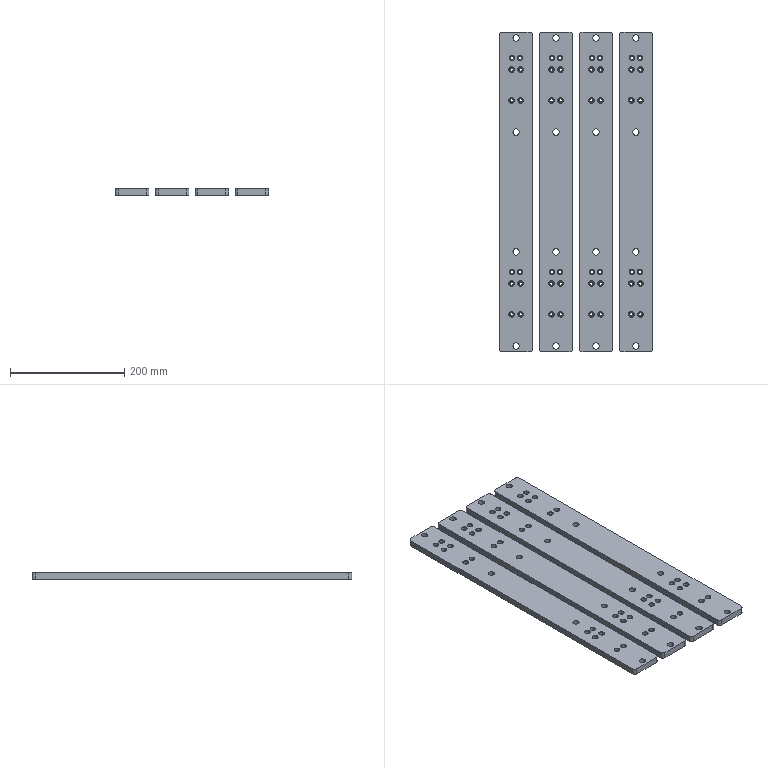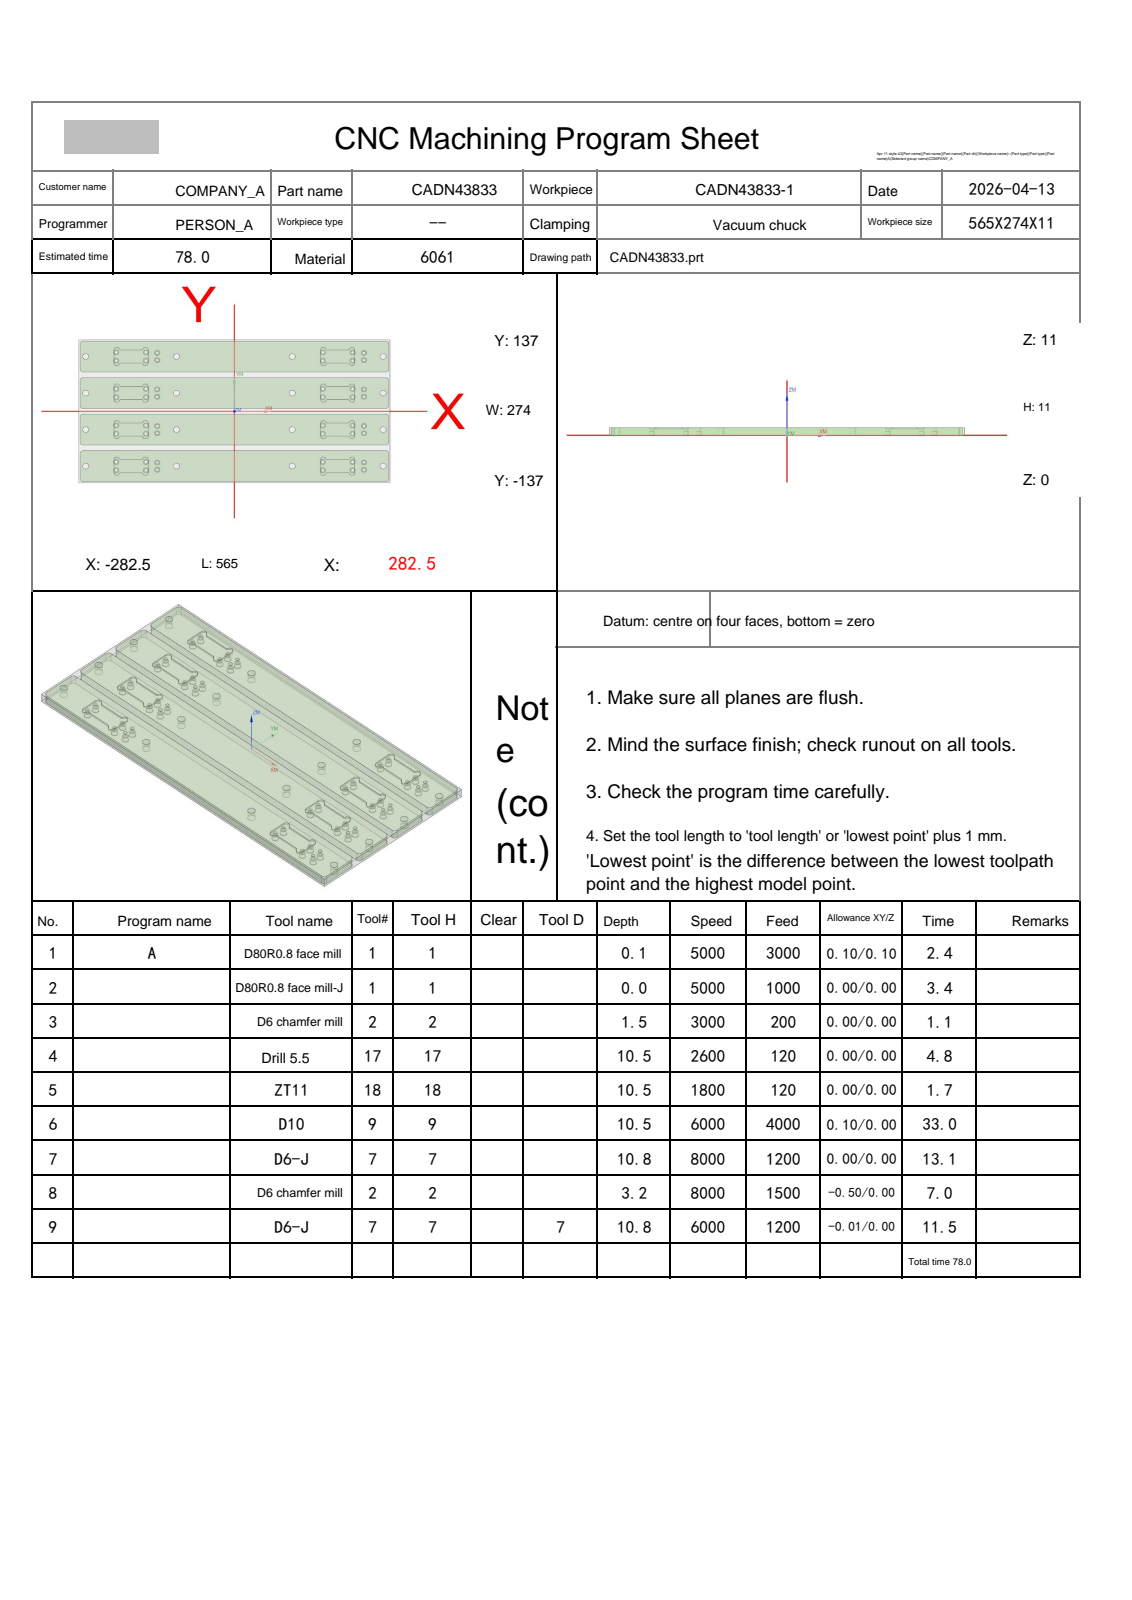NC program | NX | posted by the shop | part box 269 x 560 x 11 mm
Lines 1919 to 2898 of 6644:
N7 T07 M06
(D6-J  D=6. R=0. H=07 ce=0.30 di=0.00)
G00 G90 G54 X159.75 Y105.573 M03 S6000
G43 H07 Z31.
M08
Z10.5
G01 Y117.687 Z10.077 F1200.
X159.861 Y118.142 Z10.061
X160.089 Y118.552 Z10.044
X160.416 Y118.887 Z10.028
X160.82 Y119.124 Z10.012
X161. Y119.177 Z10.005
X161.18 Y119.231 Z9.998
X161.655 Y119.253 Z9.982
X162.12 Y119.147 Z9.965
X162.539 Y118.921 Z9.949
X162.882 Y118.59 Z9.932
X163.124 Y118.18 Z9.915
X163.27 Y117.689 Z9.897
X163.654 Y116.868 Z9.866
X164.173 Y116.125 Z9.834
X164.813 Y115.483 Z9.802
X165.553 Y114.959 Z9.771
X166.132 Y114.667 Z9.748
X166.99 Y114.383 Z9.717
X167.884 Y114.25 Z9.685
X187.5 Z9.
X206.792
G03 X211.823 Y118. I0.0 J5.25
G02 X213.5 Y119.25 I1.677 J-.5
X215.25 Y117.5 I0.0 J-1.75
G01 Y92.5
G02 X213.5 Y90.75 I-1.75 J0.0
X211.823 Y92. I0.0 J1.75
G03 X206.792 Y95.75 I-5.031 J-1.5
G01 X168.208
G03 X163.177 Y92. I0.0 J-5.25
G02 X161.5 Y90.75 I-1.677 J.5
X159.75 Y92.5 I0.0 J1.75
G01 Y117.5
G02 X161.5 Y119.25 I1.75 J0.0
X163.177 Y118. I0.0 J-1.75
G03 X168.208 Y114.25 I5.031 J1.5
G01 X187.5
Y110.05
X206.792
G03 X211.05 Y111.064 I0.0 J9.45
G01 Y98.936
G03 X206.792 Y99.95 I-4.258 J-8.436
G01 X168.208
G03 X163.95 Y98.936 I0.0 J-9.45
G01 Y111.064
G03 X168.208 Y110.05 I4.258 J8.436
G01 X187.5
Y105.85
X206.792
X206.85
Y104.15
X168.15
Y105.85
X168.208
X187.5
X188.
Y109.45
Z9.5
G00 Z31.
X159.75 Y35.573
Z10.5
G01 Y47.687 Z10.077
X159.861 Y48.142 Z10.061
X160.089 Y48.552 Z10.044
X160.416 Y48.887 Z10.028
X160.82 Y49.124 Z10.012
X161.18 Y49.231 Z9.998
X161.655 Y49.253 Z9.982
X162.12 Y49.147 Z9.965
X162.539 Y48.921 Z9.949
X162.882 Y48.59 Z9.932
X163.124 Y48.18 Z9.915
X163.27 Y47.689 Z9.897
X163.654 Y46.868 Z9.866
X164.173 Y46.125 Z9.834
X164.813 Y45.483 Z9.802
X165.553 Y44.959 Z9.771
X166.132 Y44.667 Z9.748
X166.99 Y44.383 Z9.717
X167.884 Y44.25 Z9.685
X187.5 Z9.
X206.792
G03 X211.823 Y48. I0.0 J5.25
G02 X213.5 Y49.25 I1.677 J-.5
X215.25 Y47.5 I0.0 J-1.75
G01 Y22.5
G02 X213.5 Y20.75 I-1.75 J0.0
X211.823 Y22. I0.0 J1.75
G03 X206.792 Y25.75 I-5.031 J-1.5
G01 X168.208
G03 X163.177 Y22. I0.0 J-5.25
G02 X161.5 Y20.75 I-1.677 J.5
X159.75 Y22.5 I0.0 J1.75
G01 Y47.5
G02 X161.5 Y49.25 I1.75 J0.0
X163.177 Y48. I0.0 J-1.75
G03 X168.208 Y44.25 I5.031 J1.5
G01 X187.5
Y40.05
X206.792
G03 X211.05 Y41.064 I0.0 J9.45
G01 Y28.936
G03 X206.792 Y29.95 I-4.258 J-8.436
G01 X168.208
G03 X163.95 Y28.936 I0.0 J-9.45
G01 Y41.064
G03 X168.208 Y40.05 I4.258 J8.436
G01 X187.5
Y35.85
X206.792
X206.85
Y34.15
X168.15
Y35.85
X168.208
X187.5
X188.
Y39.45
Z9.5
G00 Z31.
X159.75 Y-34.427
Z10.5
G01 Y-22.313 Z10.077
X159.861 Y-21.858 Z10.061
X160.089 Y-21.448 Z10.044
X160.416 Y-21.113 Z10.028
X160.82 Y-20.876 Z10.012
X161. Y-20.823 Z10.005
X161.18 Y-20.769 Z9.998
X161.655 Y-20.747 Z9.982
X162.12 Y-20.853 Z9.965
X162.539 Y-21.079 Z9.949
X162.882 Y-21.41 Z9.932
X163.124 Y-21.82 Z9.915
X163.27 Y-22.311 Z9.897
X163.654 Y-23.132 Z9.866
X164.173 Y-23.875 Z9.834
X164.813 Y-24.517 Z9.802
X165.553 Y-25.041 Z9.771
X166.132 Y-25.333 Z9.748
X166.99 Y-25.617 Z9.717
X167.884 Y-25.75 Z9.685
X187.5 Z9.
X206.792
G03 X211.823 Y-22. I0.0 J5.25
G02 X213.5 Y-20.75 I1.677 J-.5
X215.25 Y-22.5 I0.0 J-1.75
G01 Y-47.5
G02 X213.5 Y-49.25 I-1.75 J0.0
X211.823 Y-48. I0.0 J1.75
G03 X206.792 Y-44.25 I-5.031 J-1.5
G01 X168.208
G03 X163.177 Y-48. I0.0 J-5.25
G02 X161.5 Y-49.25 I-1.677 J.5
X159.75 Y-47.5 I0.0 J1.75
G01 Y-22.5
G02 X161.5 Y-20.75 I1.75 J0.0
X163.177 Y-22. I0.0 J-1.75
G03 X168.208 Y-25.75 I5.031 J1.5
G01 X187.5
Y-29.95
X206.792
G03 X211.05 Y-28.936 I0.0 J9.45
G01 Y-41.064
G03 X206.792 Y-40.05 I-4.258 J-8.436
G01 X168.208
G03 X163.95 Y-41.064 I0.0 J-9.45
G01 Y-28.936
G03 X168.208 Y-29.95 I4.258 J8.436
G01 X187.5
Y-34.15
X206.792
X206.85
Y-35.85
X168.15
Y-34.15
X168.208
X187.5
X188.
Y-30.55
Z9.5
G00 Z31.
X215.25 Y-105.573
Z10.5
G01 Y-117.687 Z10.077
X215.139 Y-118.142 Z10.061
X214.911 Y-118.552 Z10.044
X214.584 Y-118.887 Z10.028
X214.18 Y-119.124 Z10.012
X213.82 Y-119.231 Z9.998
X213.345 Y-119.253 Z9.982
X212.88 Y-119.147 Z9.965
X212.461 Y-118.921 Z9.949
X212.118 Y-118.59 Z9.932
X211.876 Y-118.18 Z9.915
X211.73 Y-117.689 Z9.897
X211.346 Y-116.868 Z9.866
X210.827 Y-116.125 Z9.834
X210.187 Y-115.483 Z9.802
X209.447 Y-114.959 Z9.771
X208.868 Y-114.667 Z9.748
X208.01 Y-114.383 Z9.717
X207.116 Y-114.25 Z9.685
X187.5 Z9.
X168.208
G03 X163.177 Y-118. I0.0 J-5.25
G02 X161.5 Y-119.25 I-1.677 J.5
X159.75 Y-117.5 I0.0 J1.75
G01 Y-92.5
G02 X161.5 Y-90.75 I1.75 J0.0
X163.177 Y-92. I0.0 J-1.75
G03 X168.208 Y-95.75 I5.031 J1.5
G01 X206.792
G03 X211.823 Y-92. I0.0 J5.25
G02 X213.5 Y-90.75 I1.677 J-.5
X215.25 Y-92.5 I0.0 J-1.75
G01 Y-117.5
G02 X213.5 Y-119.25 I-1.75 J0.0
X211.823 Y-118. I0.0 J1.75
G03 X206.792 Y-114.25 I-5.031 J-1.5
G01 X187.5
Y-110.05
X168.208
G03 X163.95 Y-111.064 I0.0 J-9.45
G01 Y-98.936
G03 X168.208 Y-99.95 I4.258 J8.436
G01 X206.792
G03 X211.05 Y-98.936 I0.0 J9.45
G01 Y-111.064
G03 X206.792 Y-110.05 I-4.258 J-8.436
G01 X187.5
Y-105.85
X168.208
X168.15
Y-104.15
X206.85
Y-105.85
X206.792
X187.5
X187.
Y-109.45
Z9.5
G00 Z31.
X-159.75 Y-105.573
Z10.5
G01 Y-117.687 Z10.077
X-159.861 Y-118.142 Z10.061
X-160.089 Y-118.552 Z10.044
X-160.416 Y-118.887 Z10.028
X-160.82 Y-119.124 Z10.012
X-161.18 Y-119.231 Z9.998
X-161.655 Y-119.253 Z9.982
X-162.12 Y-119.147 Z9.965
X-162.539 Y-118.921 Z9.949
X-162.882 Y-118.59 Z9.932
X-163.124 Y-118.18 Z9.915
X-163.27 Y-117.689 Z9.897
X-163.654 Y-116.868 Z9.866
X-164.173 Y-116.125 Z9.834
X-164.813 Y-115.483 Z9.802
X-165.553 Y-114.959 Z9.771
X-166.132 Y-114.667 Z9.748
X-166.99 Y-114.383 Z9.717
X-167.884 Y-114.25 Z9.685
X-187.5 Z9.
X-206.792
G03 X-211.823 Y-118. I0.0 J-5.25
G02 X-213.5 Y-119.25 I-1.677 J.5
X-215.25 Y-117.5 I0.0 J1.75
G01 Y-92.5
G02 X-213.5 Y-90.75 I1.75 J0.0
X-211.823 Y-92. I0.0 J-1.75
G03 X-206.792 Y-95.75 I5.031 J1.5
G01 X-168.208
G03 X-163.177 Y-92. I0.0 J5.25
G02 X-161.5 Y-90.75 I1.677 J-.5
X-159.75 Y-92.5 I0.0 J-1.75
G01 Y-117.5
G02 X-161.5 Y-119.25 I-1.75 J0.0
X-163.177 Y-118. I0.0 J1.75
G03 X-168.208 Y-114.25 I-5.031 J-1.5
G01 X-187.5
Y-110.05
X-206.792
G03 X-211.05 Y-111.064 I0.0 J-9.45
G01 Y-98.936
G03 X-206.792 Y-99.95 I4.258 J8.436
G01 X-168.208
G03 X-163.95 Y-98.936 I0.0 J9.45
G01 Y-111.064
G03 X-168.208 Y-110.05 I-4.258 J-8.436
G01 X-187.5
Y-105.85
X-206.792
X-206.85
Y-104.15
X-168.15
Y-105.85
X-168.208
X-187.5
X-188.
Y-109.45
Z9.5
G00 Z31.
X-159.75 Y-35.573
Z10.5
G01 Y-47.687 Z10.077
X-159.861 Y-48.142 Z10.061
X-160.089 Y-48.552 Z10.044
X-160.416 Y-48.887 Z10.028
X-160.82 Y-49.124 Z10.012
X-161.18 Y-49.231 Z9.998
X-161.655 Y-49.253 Z9.982
X-162.12 Y-49.147 Z9.965
X-162.539 Y-48.921 Z9.949
X-162.882 Y-48.59 Z9.932
X-163.124 Y-48.18 Z9.915
X-163.27 Y-47.689 Z9.897
X-163.654 Y-46.868 Z9.866
X-164.173 Y-46.125 Z9.834
X-164.813 Y-45.483 Z9.802
X-165.553 Y-44.959 Z9.771
X-166.132 Y-44.667 Z9.748
X-166.99 Y-44.383 Z9.717
X-167.884 Y-44.25 Z9.685
X-187.5 Z9.
X-206.792
G03 X-211.823 Y-48. I0.0 J-5.25
G02 X-213.5 Y-49.25 I-1.677 J.5
X-215.25 Y-47.5 I0.0 J1.75
G01 Y-22.5
G02 X-213.5 Y-20.75 I1.75 J0.0
X-211.823 Y-22. I0.0 J-1.75
G03 X-206.792 Y-25.75 I5.031 J1.5
G01 X-168.208
G03 X-163.177 Y-22. I0.0 J5.25
G02 X-161.5 Y-20.75 I1.677 J-.5
X-159.75 Y-22.5 I0.0 J-1.75
G01 Y-47.5
G02 X-161.5 Y-49.25 I-1.75 J0.0
X-163.177 Y-48. I0.0 J1.75
G03 X-168.208 Y-44.25 I-5.031 J-1.5
G01 X-187.5
Y-40.05
X-206.792
G03 X-211.05 Y-41.064 I0.0 J-9.45
G01 Y-28.936
G03 X-206.792 Y-29.95 I4.258 J8.436
G01 X-168.208
G03 X-163.95 Y-28.936 I0.0 J9.45
G01 Y-41.064
G03 X-168.208 Y-40.05 I-4.258 J-8.436
G01 X-187.5
Y-35.85
X-206.792
X-206.85
Y-34.15
X-168.15
Y-35.85
X-168.208
X-187.5
X-188.
Y-39.45
Z9.5
G00 Z31.
X-159.75 Y34.427
Z10.5
G01 Y22.313 Z10.077
X-159.861 Y21.858 Z10.061
X-160.089 Y21.448 Z10.044
X-160.416 Y21.113 Z10.028
X-160.82 Y20.876 Z10.012
X-161.18 Y20.769 Z9.998
X-161.655 Y20.747 Z9.982
X-162.12 Y20.853 Z9.965
X-162.539 Y21.079 Z9.949
X-162.882 Y21.41 Z9.932
X-163.124 Y21.82 Z9.915
X-163.27 Y22.311 Z9.897
X-163.654 Y23.132 Z9.866
X-164.173 Y23.875 Z9.834
X-164.813 Y24.517 Z9.802
X-165.553 Y25.041 Z9.771
X-166.132 Y25.333 Z9.748
X-166.99 Y25.617 Z9.717
X-167.884 Y25.75 Z9.685
X-187.5 Z9.
X-206.792
G03 X-211.823 Y22. I0.0 J-5.25
G02 X-213.5 Y20.75 I-1.677 J.5
X-215.25 Y22.5 I0.0 J1.75
G01 Y47.5
G02 X-213.5 Y49.25 I1.75 J0.0
X-211.823 Y48. I0.0 J-1.75
G03 X-206.792 Y44.25 I5.031 J1.5
G01 X-168.208
G03 X-163.177 Y48. I0.0 J5.25
G02 X-161.5 Y49.25 I1.677 J-.5
X-159.75 Y47.5 I0.0 J-1.75
G01 Y22.5
G02 X-161.5 Y20.75 I-1.75 J0.0
X-163.177 Y22. I0.0 J1.75
G03 X-168.208 Y25.75 I-5.031 J-1.5
G01 X-187.5
Y29.95
X-206.792
G03 X-211.05 Y28.936 I0.0 J-9.45
G01 Y41.064
G03 X-206.792 Y40.05 I4.258 J8.436
G01 X-168.208
G03 X-163.95 Y41.064 I0.0 J9.45
G01 Y28.936
G03 X-168.208 Y29.95 I-4.258 J-8.436
G01 X-187.5
Y34.15
X-206.792
X-206.85
Y35.85
X-168.15
Y34.15
X-168.208
X-187.5
X-188.
Y30.55
Z9.5
G00 Z31.
X-215.25 Y105.573
Z10.5
G01 Y117.687 Z10.077
X-215.139 Y118.142 Z10.061
X-214.911 Y118.552 Z10.044
X-214.584 Y118.887 Z10.028
X-214.18 Y119.124 Z10.012
X-213.82 Y119.231 Z9.998
X-213.345 Y119.253 Z9.982
X-212.88 Y119.147 Z9.965
X-212.461 Y118.921 Z9.949
X-212.118 Y118.59 Z9.932
X-211.876 Y118.18 Z9.915
X-211.73 Y117.689 Z9.897
X-211.346 Y116.868 Z9.866
X-210.827 Y116.125 Z9.834
X-210.187 Y115.483 Z9.802
X-209.447 Y114.959 Z9.771
X-208.868 Y114.667 Z9.748
X-208.01 Y114.383 Z9.717
X-207.116 Y114.25 Z9.685
X-187.5 Z9.
X-168.208
G03 X-163.177 Y118. I0.0 J5.25
G02 X-161.5 Y119.25 I1.677 J-.5
X-159.75 Y117.5 I0.0 J-1.75
G01 Y92.5
G02 X-161.5 Y90.75 I-1.75 J0.0
X-163.177 Y92. I0.0 J1.75
G03 X-168.208 Y95.75 I-5.031 J-1.5
G01 X-206.792
G03 X-211.823 Y92. I0.0 J-5.25
G02 X-213.5 Y90.75 I-1.677 J.5
X-215.25 Y92.5 I0.0 J1.75
G01 Y117.5
G02 X-213.5 Y119.25 I1.75 J0.0
X-211.823 Y118. I0.0 J-1.75
G03 X-206.792 Y114.25 I5.031 J1.5
G01 X-187.5
Y110.05
X-168.208
G03 X-163.95 Y111.064 I0.0 J9.45
G01 Y98.936
G03 X-168.208 Y99.95 I-4.258 J-8.436
G01 X-206.792
G03 X-211.05 Y98.936 I0.0 J-9.45
G01 Y111.064
G03 X-206.792 Y110.05 I4.258 J8.436
G01 X-187.5
Y105.85
X-168.208
X-168.15
Y104.15
X-206.85
Y105.85
X-206.792
X-187.5
X-187.
Y109.45
Z9.5
G00 Z31.
G00 G90 X-268.18 Y103.339 M03 S8000
Z31.
Z11.5
G01 X-268.119 Y103.399 Z11.496 F600.
X-267.888 Y103.72 Z11.475
X-267.71 Y104.074 Z11.454
X-267.592 Y104.451 Z11.433
X-267.535 Y104.843 Z11.413
Y105.157 Z11.396
X-267.592 Y105.549 Z11.375
X-267.71 Y105.926 Z11.355
X-267.888 Y106.28 Z11.334
X-268.119 Y106.601 Z11.313
X-268.399 Y106.881 Z11.292
X-268.72 Y107.112 Z11.272
X-269.074 Y107.29 Z11.251
X-269.451 Y107.408 Z11.23
X-269.843 Y107.465 Z11.209
X-270.157 Z11.193
X-270.593 Y107.398 Z11.17
X-271.009 Y107.254 Z11.147
X-271.394 Y107.039 Z11.124
X-271.734 Y106.759 Z11.101
X-272.019 Y106.423 Z11.078
X-272.24 Y106.041 Z11.054
X-272.389 Y105.627 Z11.031
X-272.462 Y105.192 Z11.008
X-272.465 Y105.035 Z11.
G41 D07
X-272.5 Y105.
G03 X-270. Y102.5 Z10.877 I2.5 J0.0
X-267.5 Y105. Z10.755 I0.0 J2.5
X-270. Y107.5 Z10.632 I-2.5 J0.0
X-272.5 Y105. Z10.509 I0.0 J-2.5
X-270. Y102.5 Z10.386 I2.5 J0.0
X-267.5 Y105. Z10.264 I0.0 J2.5
X-270. Y107.5 Z10.141 I-2.5 J0.0
X-272.5 Y105. Z10.018 I0.0 J-2.5
X-270. Y102.5 Z9.895 I2.5 J0.0
X-267.5 Y105. Z9.773 I0.0 J2.5
X-270. Y107.5 Z9.65 I-2.5 J0.0
X-272.5 Y105. Z9.527 I0.0 J-2.5
X-270. Y102.5 Z9.405 I2.5 J0.0
X-267.5 Y105. Z9.282 I0.0 J2.5
X-270. Y107.5 Z9.159 I-2.5 J0.0
X-272.5 Y105. Z9.036 I0.0 J-2.5
X-270. Y102.5 Z8.914 I2.5 J0.0
X-267.5 Y105. Z8.791 I0.0 J2.5
X-270. Y107.5 Z8.668 I-2.5 J0.0
X-272.5 Y105. Z8.545 I0.0 J-2.5
X-270. Y102.5 Z8.423 I2.5 J0.0
X-267.5 Y105. Z8.3 I0.0 J2.5
X-270. Y107.5 Z8.177 I-2.5 J0.0
X-272.5 Y105. Z8.055 I0.0 J-2.5
X-270. Y102.5 Z7.932 I2.5 J0.0
X-267.5 Y105. Z7.809 I0.0 J2.5
X-270. Y107.5 Z7.686 I-2.5 J0.0
X-272.5 Y105. Z7.564 I0.0 J-2.5
X-270. Y102.5 Z7.441 I2.5 J0.0
X-267.5 Y105. Z7.318 I0.0 J2.5
X-270. Y107.5 Z7.195 I-2.5 J0.0
X-272.5 Y105. Z7.073 I0.0 J-2.5
X-270. Y102.5 Z6.95 I2.5 J0.0
X-267.5 Y105. Z6.827 I0.0 J2.5
X-270. Y107.5 Z6.705 I-2.5 J0.0
X-272.5 Y105. Z6.582 I0.0 J-2.5
X-270. Y102.5 Z6.459 I2.5 J0.0
X-267.5 Y105. Z6.336 I0.0 J2.5
X-270. Y107.5 Z6.214 I-2.5 J0.0
X-272.5 Y105. Z6.091 I0.0 J-2.5
X-270. Y102.5 Z5.968 I2.5 J0.0
X-267.5 Y105. Z5.845 I0.0 J2.5
X-270. Y107.5 Z5.723 I-2.5 J0.0
X-272.5 Y105. Z5.6 I0.0 J-2.5
X-270. Y102.5 Z5.477 I2.5 J0.0
X-267.5 Y105. Z5.355 I0.0 J2.5
X-270. Y107.5 Z5.232 I-2.5 J0.0
X-272.5 Y105. Z5.109 I0.0 J-2.5
X-270. Y102.5 Z4.986 I2.5 J0.0
X-267.5 Y105. Z4.864 I0.0 J2.5
X-270. Y107.5 Z4.741 I-2.5 J0.0
X-272.5 Y105. Z4.618 I0.0 J-2.5
X-270. Y102.5 Z4.495 I2.5 J0.0
X-267.5 Y105. Z4.373 I0.0 J2.5
X-270. Y107.5 Z4.25 I-2.5 J0.0
X-272.5 Y105. Z4.127 I0.0 J-2.5
X-270. Y102.5 Z4.005 I2.5 J0.0
X-267.5 Y105. Z3.882 I0.0 J2.5
X-270. Y107.5 Z3.759 I-2.5 J0.0
X-272.5 Y105. Z3.636 I0.0 J-2.5
X-270. Y102.5 Z3.514 I2.5 J0.0
X-267.5 Y105. Z3.391 I0.0 J2.5
X-270. Y107.5 Z3.268 I-2.5 J0.0
X-272.5 Y105. Z3.145 I0.0 J-2.5
X-270. Y102.5 Z3.023 I2.5 J0.0
X-267.5 Y105. Z2.9 I0.0 J2.5
X-270. Y107.5 Z2.777 I-2.5 J0.0
X-272.5 Y105. Z2.655 I0.0 J-2.5
X-270. Y102.5 Z2.532 I2.5 J0.0
X-267.5 Y105. Z2.409 I0.0 J2.5
X-270. Y107.5 Z2.286 I-2.5 J0.0
X-272.5 Y105. Z2.164 I0.0 J-2.5
X-270. Y102.5 Z2.041 I2.5 J0.0
X-267.5 Y105. Z1.918 I0.0 J2.5
X-270. Y107.5 Z1.795 I-2.5 J0.0
X-272.5 Y105. Z1.673 I0.0 J-2.5
X-270. Y102.5 Z1.55 I2.5 J0.0
X-267.5 Y105. Z1.427 I0.0 J2.5
X-270. Y107.5 Z1.305 I-2.5 J0.0
X-272.5 Y105. Z1.182 I0.0 J-2.5
X-270. Y102.5 Z1.059 I2.5 J0.0
X-267.5 Y105. Z.936 I0.0 J2.5
X-270. Y107.5 Z.814 I-2.5 J0.0
X-272.5 Y105. Z.691 I0.0 J-2.5
X-270. Y102.5 Z.568 I2.5 J0.0
X-267.5 Y105. Z.445 I0.0 J2.5
X-270. Y107.5 Z.323 I-2.5 J0.0
X-272.5 Y105. Z.2 I0.0 J-2.5
X-270. Y102.5 I2.5 J0.0
X-267.5 Y105. I0.0 J2.5
X-270. Y107.5 I-2.5 J0.0
X-272.5 Y105. I0.0 J-2.5
X-272.468 Y104.602 I2.5 J0.0
G01 X-272.461 Y104.575
X-272.438 Y104.558
X-272.411 Y104.56
G40 X-272.361 Y104.568
Z1.2
G00 Z31.
X-268.18 Y33.339
Z11.5
G01 X-268.119 Y33.399 Z11.496
X-267.888 Y33.72 Z11.475
X-267.71 Y34.074 Z11.454
X-267.592 Y34.451 Z11.433
X-267.535 Y34.843 Z11.413
Y35.157 Z11.396
X-267.592 Y35.549 Z11.375
X-267.71 Y35.926 Z11.355
X-267.888 Y36.28 Z11.334
X-268.119 Y36.601 Z11.313
X-268.399 Y36.881 Z11.292
X-268.72 Y37.112 Z11.272
X-269.074 Y37.29 Z11.251
X-269.451 Y37.408 Z11.23
X-269.843 Y37.465 Z11.209
X-270.157 Z11.193
X-270.593 Y37.398 Z11.17
X-271.009 Y37.254 Z11.147
X-271.394 Y37.039 Z11.124
X-271.734 Y36.759 Z11.101
X-272.019 Y36.423 Z11.078
X-272.24 Y36.041 Z11.054
X-272.389 Y35.627 Z11.031
X-272.462 Y35.192 Z11.008
X-272.465 Y35.035 Z11.
G41 D07
X-272.5 Y35.
G03 X-270. Y32.5 Z10.877 I2.5 J0.0
X-267.5 Y35. Z10.755 I0.0 J2.5
X-270. Y37.5 Z10.632 I-2.5 J0.0
X-272.5 Y35. Z10.509 I0.0 J-2.5
X-270. Y32.5 Z10.386 I2.5 J0.0
X-267.5 Y35. Z10.264 I0.0 J2.5
X-270. Y37.5 Z10.141 I-2.5 J0.0
X-272.5 Y35. Z10.018 I0.0 J-2.5
X-270. Y32.5 Z9.895 I2.5 J0.0
X-267.5 Y35. Z9.773 I0.0 J2.5
X-270. Y37.5 Z9.65 I-2.5 J0.0
X-272.5 Y35. Z9.527 I0.0 J-2.5
X-270. Y32.5 Z9.405 I2.5 J0.0
X-267.5 Y35. Z9.282 I0.0 J2.5
X-270. Y37.5 Z9.159 I-2.5 J0.0
X-272.5 Y35. Z9.036 I0.0 J-2.5
X-270. Y32.5 Z8.914 I2.5 J0.0
X-267.5 Y35. Z8.791 I0.0 J2.5
X-270. Y37.5 Z8.668 I-2.5 J0.0
X-272.5 Y35. Z8.545 I0.0 J-2.5
X-270. Y32.5 Z8.423 I2.5 J0.0
X-267.5 Y35. Z8.3 I0.0 J2.5
X-270. Y37.5 Z8.177 I-2.5 J0.0
X-272.5 Y35. Z8.055 I0.0 J-2.5
X-270. Y32.5 Z7.932 I2.5 J0.0
X-267.5 Y35. Z7.809 I0.0 J2.5
X-270. Y37.5 Z7.686 I-2.5 J0.0
X-272.5 Y35. Z7.564 I0.0 J-2.5
X-270. Y32.5 Z7.441 I2.5 J0.0
X-267.5 Y35. Z7.318 I0.0 J2.5
X-270. Y37.5 Z7.195 I-2.5 J0.0
X-272.5 Y35. Z7.073 I0.0 J-2.5
X-270. Y32.5 Z6.95 I2.5 J0.0
X-267.5 Y35. Z6.827 I0.0 J2.5
X-270. Y37.5 Z6.705 I-2.5 J0.0
X-272.5 Y35. Z6.582 I0.0 J-2.5
X-270. Y32.5 Z6.459 I2.5 J0.0
X-267.5 Y35. Z6.336 I0.0 J2.5
X-270. Y37.5 Z6.214 I-2.5 J0.0
X-272.5 Y35. Z6.091 I0.0 J-2.5
X-270. Y32.5 Z5.968 I2.5 J0.0
X-267.5 Y35. Z5.845 I0.0 J2.5
X-270. Y37.5 Z5.723 I-2.5 J0.0
X-272.5 Y35. Z5.6 I0.0 J-2.5
X-270. Y32.5 Z5.477 I2.5 J0.0
X-267.5 Y35. Z5.355 I0.0 J2.5
X-270. Y37.5 Z5.232 I-2.5 J0.0
X-272.5 Y35. Z5.109 I0.0 J-2.5
X-270. Y32.5 Z4.986 I2.5 J0.0
X-267.5 Y35. Z4.864 I0.0 J2.5
X-270. Y37.5 Z4.741 I-2.5 J0.0
X-272.5 Y35. Z4.618 I0.0 J-2.5
X-270. Y32.5 Z4.495 I2.5 J0.0
X-267.5 Y35. Z4.373 I0.0 J2.5
X-270. Y37.5 Z4.25 I-2.5 J0.0
X-272.5 Y35. Z4.127 I0.0 J-2.5
X-270. Y32.5 Z4.005 I2.5 J0.0
X-267.5 Y35. Z3.882 I0.0 J2.5
X-270. Y37.5 Z3.759 I-2.5 J0.0
X-272.5 Y35. Z3.636 I0.0 J-2.5
X-270. Y32.5 Z3.514 I2.5 J0.0
X-267.5 Y35. Z3.391 I0.0 J2.5
X-270. Y37.5 Z3.268 I-2.5 J0.0
X-272.5 Y35. Z3.145 I0.0 J-2.5
X-270. Y32.5 Z3.023 I2.5 J0.0
X-267.5 Y35. Z2.9 I0.0 J2.5
X-270. Y37.5 Z2.777 I-2.5 J0.0
X-272.5 Y35. Z2.655 I0.0 J-2.5
X-270. Y32.5 Z2.532 I2.5 J0.0
X-267.5 Y35. Z2.409 I0.0 J2.5
X-270. Y37.5 Z2.286 I-2.5 J0.0
X-272.5 Y35. Z2.164 I0.0 J-2.5
X-270. Y32.5 Z2.041 I2.5 J0.0
X-267.5 Y35. Z1.918 I0.0 J2.5
X-270. Y37.5 Z1.795 I-2.5 J0.0
X-272.5 Y35. Z1.673 I0.0 J-2.5
X-270. Y32.5 Z1.55 I2.5 J0.0
X-267.5 Y35. Z1.427 I0.0 J2.5
X-270. Y37.5 Z1.305 I-2.5 J0.0
X-272.5 Y35. Z1.182 I0.0 J-2.5
X-270. Y32.5 Z1.059 I2.5 J0.0
X-267.5 Y35. Z.936 I0.0 J2.5
X-270. Y37.5 Z.814 I-2.5 J0.0
X-272.5 Y35. Z.691 I0.0 J-2.5
X-270. Y32.5 Z.568 I2.5 J0.0
X-267.5 Y35. Z.445 I0.0 J2.5
X-270. Y37.5 Z.323 I-2.5 J0.0
X-272.5 Y35. Z.2 I0.0 J-2.5
X-270. Y32.5 I2.5 J0.0
X-267.5 Y35. I0.0 J2.5
X-270. Y37.5 I-2.5 J0.0
X-272.5 Y35. I0.0 J-2.5
X-272.468 Y34.602 I2.5 J0.0
G01 X-272.461 Y34.575
X-272.438 Y34.558
X-272.411 Y34.56
G40 X-272.361 Y34.568
Z1.2
G00 Z31.
X-268.18 Y-36.661
Z11.5
G01 X-268.119 Y-36.601 Z11.496
X-267.888 Y-36.28 Z11.475
X-267.71 Y-35.926 Z11.454
X-267.592 Y-35.549 Z11.433
X-267.535 Y-35.157 Z11.413
Y-34.843 Z11.396
X-267.592 Y-34.451 Z11.375
X-267.71 Y-34.074 Z11.355
X-267.888 Y-33.72 Z11.334
X-268.119 Y-33.399 Z11.313
X-268.399 Y-33.119 Z11.292
X-268.72 Y-32.888 Z11.272
X-269.074 Y-32.71 Z11.251
X-269.451 Y-32.592 Z11.23
X-269.843 Y-32.535 Z11.209
X-270.157 Z11.193
X-270.593 Y-32.602 Z11.17
X-271.009 Y-32.746 Z11.147
X-271.394 Y-32.961 Z11.124
X-271.734 Y-33.241 Z11.101
X-272.019 Y-33.577 Z11.078
X-272.24 Y-33.959 Z11.054
X-272.389 Y-34.373 Z11.031
X-272.462 Y-34.808 Z11.008
X-272.465 Y-34.965 Z11.
G41 D07
X-272.5 Y-35.
G03 X-270. Y-37.5 Z10.877 I2.5 J0.0
X-267.5 Y-35. Z10.755 I0.0 J2.5
X-270. Y-32.5 Z10.632 I-2.5 J0.0
X-272.5 Y-35. Z10.509 I0.0 J-2.5
X-270. Y-37.5 Z10.386 I2.5 J0.0
X-267.5 Y-35. Z10.264 I0.0 J2.5
X-270. Y-32.5 Z10.141 I-2.5 J0.0
X-272.5 Y-35. Z10.018 I0.0 J-2.5
X-270. Y-37.5 Z9.895 I2.5 J0.0
X-267.5 Y-35. Z9.773 I0.0 J2.5
X-270. Y-32.5 Z9.65 I-2.5 J0.0
X-272.5 Y-35. Z9.527 I0.0 J-2.5
X-270. Y-37.5 Z9.405 I2.5 J0.0
X-267.5 Y-35. Z9.282 I0.0 J2.5
X-270. Y-32.5 Z9.159 I-2.5 J0.0
X-272.5 Y-35. Z9.036 I0.0 J-2.5
X-270. Y-37.5 Z8.914 I2.5 J0.0
X-267.5 Y-35. Z8.791 I0.0 J2.5
X-270. Y-32.5 Z8.668 I-2.5 J0.0
X-272.5 Y-35. Z8.545 I0.0 J-2.5
X-270. Y-37.5 Z8.423 I2.5 J0.0
X-267.5 Y-35. Z8.3 I0.0 J2.5
X-270. Y-32.5 Z8.177 I-2.5 J0.0
X-272.5 Y-35. Z8.055 I0.0 J-2.5
X-270. Y-37.5 Z7.932 I2.5 J0.0
X-267.5 Y-35. Z7.809 I0.0 J2.5
X-270. Y-32.5 Z7.686 I-2.5 J0.0
X-272.5 Y-35. Z7.564 I0.0 J-2.5
X-270. Y-37.5 Z7.441 I2.5 J0.0
X-267.5 Y-35. Z7.318 I0.0 J2.5
X-270. Y-32.5 Z7.195 I-2.5 J0.0
X-272.5 Y-35. Z7.073 I0.0 J-2.5
X-270. Y-37.5 Z6.95 I2.5 J0.0
X-267.5 Y-35. Z6.827 I0.0 J2.5
X-270. Y-32.5 Z6.705 I-2.5 J0.0
X-272.5 Y-35. Z6.582 I0.0 J-2.5
X-270. Y-37.5 Z6.459 I2.5 J0.0
X-267.5 Y-35. Z6.336 I0.0 J2.5
X-270. Y-32.5 Z6.214 I-2.5 J0.0
X-272.5 Y-35. Z6.091 I0.0 J-2.5
X-270. Y-37.5 Z5.968 I2.5 J0.0
X-267.5 Y-35. Z5.845 I0.0 J2.5
X-270. Y-32.5 Z5.723 I-2.5 J0.0
X-272.5 Y-35. Z5.6 I0.0 J-2.5
X-270. Y-37.5 Z5.477 I2.5 J0.0
X-267.5 Y-35. Z5.355 I0.0 J2.5
X-270. Y-32.5 Z5.232 I-2.5 J0.0
X-272.5 Y-35. Z5.109 I0.0 J-2.5
X-270. Y-37.5 Z4.986 I2.5 J0.0
X-267.5 Y-35. Z4.864 I0.0 J2.5
X-270. Y-32.5 Z4.741 I-2.5 J0.0
X-272.5 Y-35. Z4.618 I0.0 J-2.5
X-270. Y-37.5 Z4.495 I2.5 J0.0
X-267.5 Y-35. Z4.373 I0.0 J2.5
X-270. Y-32.5 Z4.25 I-2.5 J0.0
X-272.5 Y-35. Z4.127 I0.0 J-2.5
X-270. Y-37.5 Z4.005 I2.5 J0.0
X-267.5 Y-35. Z3.882 I0.0 J2.5
X-270. Y-32.5 Z3.759 I-2.5 J0.0
X-272.5 Y-35. Z3.636 I0.0 J-2.5
X-270. Y-37.5 Z3.514 I2.5 J0.0
X-267.5 Y-35. Z3.391 I0.0 J2.5
X-270. Y-32.5 Z3.268 I-2.5 J0.0
X-272.5 Y-35. Z3.145 I0.0 J-2.5
X-270. Y-37.5 Z3.023 I2.5 J0.0
X-267.5 Y-35. Z2.9 I0.0 J2.5
X-270. Y-32.5 Z2.777 I-2.5 J0.0
X-272.5 Y-35. Z2.655 I0.0 J-2.5
X-270. Y-37.5 Z2.532 I2.5 J0.0
X-267.5 Y-35. Z2.409 I0.0 J2.5
X-270. Y-32.5 Z2.286 I-2.5 J0.0
X-272.5 Y-35. Z2.164 I0.0 J-2.5
X-270. Y-37.5 Z2.041 I2.5 J0.0
X-267.5 Y-35. Z1.918 I0.0 J2.5
X-270. Y-32.5 Z1.795 I-2.5 J0.0
X-272.5 Y-35. Z1.673 I0.0 J-2.5
X-270. Y-37.5 Z1.55 I2.5 J0.0
X-267.5 Y-35. Z1.427 I0.0 J2.5
X-270. Y-32.5 Z1.305 I-2.5 J0.0
X-272.5 Y-35. Z1.182 I0.0 J-2.5
X-270. Y-37.5 Z1.059 I2.5 J0.0
X-267.5 Y-35. Z.936 I0.0 J2.5
X-270. Y-32.5 Z.814 I-2.5 J0.0
X-272.5 Y-35. Z.691 I0.0 J-2.5
X-270. Y-37.5 Z.568 I2.5 J0.0
X-267.5 Y-35. Z.445 I0.0 J2.5
X-270. Y-32.5 Z.323 I-2.5 J0.0
X-272.5 Y-35. Z.2 I0.0 J-2.5
X-270. Y-37.5 I2.5 J0.0
X-267.5 Y-35. I0.0 J2.5
X-270. Y-32.5 I-2.5 J0.0
X-272.5 Y-35. I0.0 J-2.5
X-272.468 Y-35.398 I2.5 J0.0
G01 X-272.461 Y-35.425
X-272.438 Y-35.442
X-272.411 Y-35.44
G40 X-272.361 Y-35.432
Z1.2
G00 Z31.
X-268.18 Y-106.661
Z11.5
G01 X-268.119 Y-106.601 Z11.496
X-267.888 Y-106.28 Z11.475
X-267.71 Y-105.926 Z11.454
X-267.592 Y-105.549 Z11.433
X-267.535 Y-105.157 Z11.413
Y-104.843 Z11.396
X-267.592 Y-104.451 Z11.375
X-267.71 Y-104.074 Z11.355
X-267.888 Y-103.72 Z11.334
X-268.119 Y-103.399 Z11.313
X-268.399 Y-103.119 Z11.292
X-268.72 Y-102.888 Z11.272
X-269.074 Y-102.71 Z11.251
X-269.451 Y-102.592 Z11.23
X-269.843 Y-102.535 Z11.209
X-270.157 Z11.193
X-270.593 Y-102.602 Z11.17
X-271.009 Y-102.746 Z11.147
X-271.394 Y-102.961 Z11.124
X-271.734 Y-103.241 Z11.101
X-272.019 Y-103.577 Z11.078
X-272.24 Y-103.959 Z11.054
X-272.389 Y-104.373 Z11.031
X-272.462 Y-104.808 Z11.008
X-272.465 Y-104.965 Z11.
G41 D07
X-272.5 Y-105.
G03 X-270. Y-107.5 Z10.877 I2.5 J0.0
X-267.5 Y-105. Z10.755 I0.0 J2.5
X-270. Y-102.5 Z10.632 I-2.5 J0.0
X-272.5 Y-105. Z10.509 I0.0 J-2.5
X-270. Y-107.5 Z10.386 I2.5 J0.0
X-267.5 Y-105. Z10.264 I0.0 J2.5
X-270. Y-102.5 Z10.141 I-2.5 J0.0
X-272.5 Y-105. Z10.018 I0.0 J-2.5
X-270. Y-107.5 Z9.895 I2.5 J0.0
X-267.5 Y-105. Z9.773 I0.0 J2.5
X-270. Y-102.5 Z9.65 I-2.5 J0.0
X-272.5 Y-105. Z9.527 I0.0 J-2.5
X-270. Y-107.5 Z9.405 I2.5 J0.0
X-267.5 Y-105. Z9.282 I0.0 J2.5
X-270. Y-102.5 Z9.159 I-2.5 J0.0
X-272.5 Y-105. Z9.036 I0.0 J-2.5
X-270. Y-107.5 Z8.914 I2.5 J0.0
X-267.5 Y-105. Z8.791 I0.0 J2.5
X-270. Y-102.5 Z8.668 I-2.5 J0.0
X-272.5 Y-105. Z8.545 I0.0 J-2.5
X-270. Y-107.5 Z8.423 I2.5 J0.0
X-267.5 Y-105. Z8.3 I0.0 J2.5
X-270. Y-102.5 Z8.177 I-2.5 J0.0
X-272.5 Y-105. Z8.055 I0.0 J-2.5
X-270. Y-107.5 Z7.932 I2.5 J0.0
X-267.5 Y-105. Z7.809 I0.0 J2.5
X-270. Y-102.5 Z7.686 I-2.5 J0.0
X-272.5 Y-105. Z7.564 I0.0 J-2.5
X-270. Y-107.5 Z7.441 I2.5 J0.0
X-267.5 Y-105. Z7.318 I0.0 J2.5
X-270. Y-102.5 Z7.195 I-2.5 J0.0
X-272.5 Y-105. Z7.073 I0.0 J-2.5
X-270. Y-107.5 Z6.95 I2.5 J0.0
X-267.5 Y-105. Z6.827 I0.0 J2.5
X-270. Y-102.5 Z6.705 I-2.5 J0.0
X-272.5 Y-105. Z6.582 I0.0 J-2.5
X-270. Y-107.5 Z6.459 I2.5 J0.0
X-267.5 Y-105. Z6.336 I0.0 J2.5
X-270. Y-102.5 Z6.214 I-2.5 J0.0
X-272.5 Y-105. Z6.091 I0.0 J-2.5
X-270. Y-107.5 Z5.968 I2.5 J0.0
X-267.5 Y-105. Z5.845 I0.0 J2.5
X-270. Y-102.5 Z5.723 I-2.5 J0.0
X-272.5 Y-105. Z5.6 I0.0 J-2.5
X-270. Y-107.5 Z5.477 I2.5 J0.0
X-267.5 Y-105. Z5.355 I0.0 J2.5
X-270. Y-102.5 Z5.232 I-2.5 J0.0
X-272.5 Y-105. Z5.109 I0.0 J-2.5
X-270. Y-107.5 Z4.986 I2.5 J0.0
X-267.5 Y-105. Z4.864 I0.0 J2.5
X-270. Y-102.5 Z4.741 I-2.5 J0.0
X-272.5 Y-105. Z4.618 I0.0 J-2.5
X-270. Y-107.5 Z4.495 I2.5 J0.0
X-267.5 Y-105. Z4.373 I0.0 J2.5
X-270. Y-102.5 Z4.25 I-2.5 J0.0
X-272.5 Y-105. Z4.127 I0.0 J-2.5
X-270. Y-107.5 Z4.005 I2.5 J0.0
X-267.5 Y-105. Z3.882 I0.0 J2.5
X-270. Y-102.5 Z3.759 I-2.5 J0.0
X-272.5 Y-105. Z3.636 I0.0 J-2.5
X-270. Y-107.5 Z3.514 I2.5 J0.0
X-267.5 Y-105. Z3.391 I0.0 J2.5
X-270. Y-102.5 Z3.268 I-2.5 J0.0
X-272.5 Y-105. Z3.145 I0.0 J-2.5
X-270. Y-107.5 Z3.023 I2.5 J0.0
X-267.5 Y-105. Z2.9 I0.0 J2.5
X-270. Y-102.5 Z2.777 I-2.5 J0.0
X-272.5 Y-105. Z2.655 I0.0 J-2.5
X-270. Y-107.5 Z2.532 I2.5 J0.0
X-267.5 Y-105. Z2.409 I0.0 J2.5
X-270. Y-102.5 Z2.286 I-2.5 J0.0
X-272.5 Y-105. Z2.164 I0.0 J-2.5